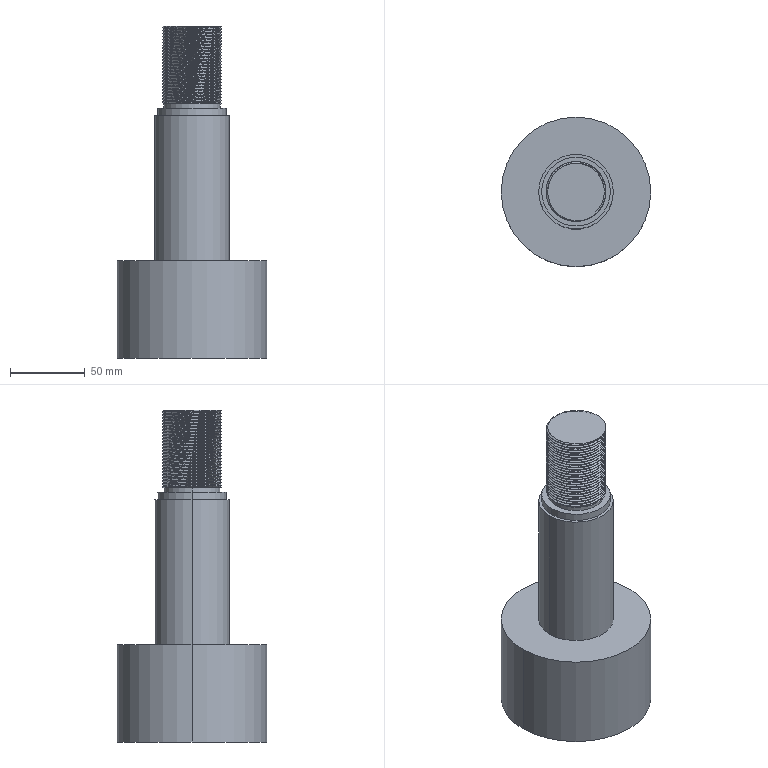Part | SolidWorks | features BaseBody 1 | 1 solid | 70 faces | box 100 x 100 x 222 mm | volume 774018 mm3 | cylinder 61 | plane 6 | spline 3 | commonest cylinder face diameters 40 x53 37.5 x2 46 x2 50 x2 100 x2